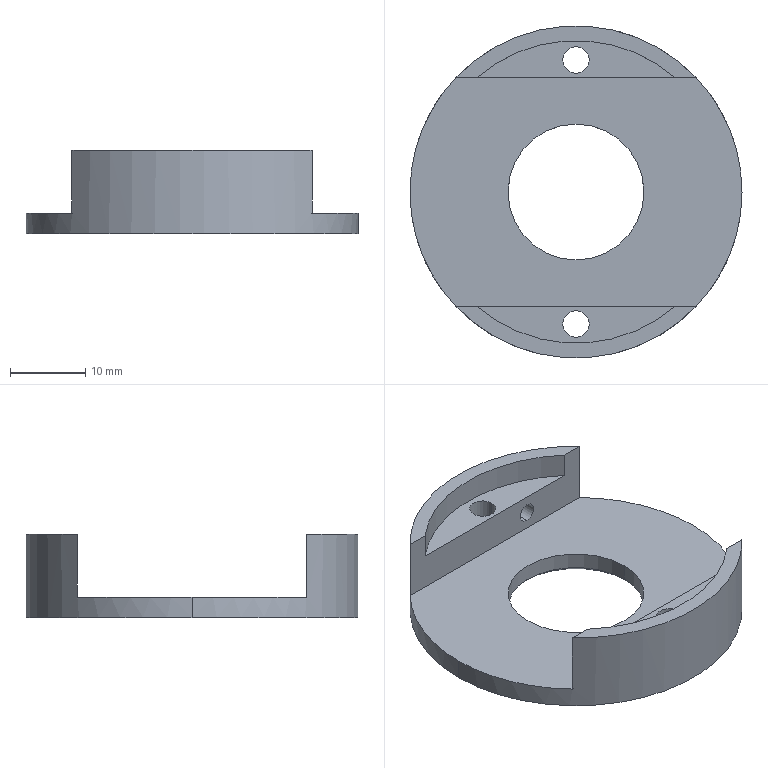Part | SolidWorks | features ICE 7, Chamfer 2, CirPattern 1, Extrusion 1 | 1 solid | 26 faces | box 44 x 44 x 11 mm | volume 5108 mm3 | cylinder 12 | plane 8 | cone 6 | commonest cylinder face diameters 3.5 x4 2.5 x2 18 x2 40.1 x2 44 x2
STEP:
#1=CARTESIAN_POINT('',(6.,21.166,6.45));
#2=VERTEX_POINT('',#1);
#3=CARTESIAN_POINT('',(6.,21.166,3.95));
#4=VERTEX_POINT('',#3);
#5=CARTESIAN_POINT('',(6.,21.166,6.45));
#6=CARTESIAN_POINT('',(5.841,21.211,6.45));
#7=CARTESIAN_POINT('',(5.679,21.255,6.419));
#8=CARTESIAN_POINT('',(5.381,21.332,6.298));
#9=CARTESIAN_POINT('',(5.241,21.367,6.207));
#10=CARTESIAN_POINT('',(5.009,21.423,5.979));
#11=CARTESIAN_POINT('',(4.913,21.444,5.839));
#12=CARTESIAN_POINT('',(4.817,21.466,5.611));
#13=CARTESIAN_POINT('',(4.792,21.472,5.53));
#14=CARTESIAN_POINT('',(4.759,21.479,5.368));
#15=CARTESIAN_POINT('',(4.75,21.481,5.285));
#16=CARTESIAN_POINT('',(4.75,21.481,5.035));
#17=CARTESIAN_POINT('',(4.783,21.474,4.87));
#18=CARTESIAN_POINT('',(4.88,21.452,4.639));
#19=CARTESIAN_POINT('',(4.919,21.443,4.567));
#20=CARTESIAN_POINT('',(5.011,21.422,4.431));
#21=CARTESIAN_POINT('',(5.065,21.409,4.367));
#22=CARTESIAN_POINT('',(5.24,21.367,4.194));
#23=CARTESIAN_POINT('',(5.379,21.333,4.103));
#24=CARTESIAN_POINT('',(5.677,21.255,3.982));
#25=CARTESIAN_POINT('',(5.839,21.212,3.95));
#26=CARTESIAN_POINT('',(6.,21.166,3.95));
#27=B_SPLINE_CURVE_WITH_KNOTS('',3,(#5,#6,#7,#8,#9,#10,#11,#12,#13,#14,#15,#16,#17,#18,#19,#20,#21,#22,#23,#24,#25,#26),.UNSPECIFIED.,.F.,.F.,(4,2,2,2,2,2,2,2,2,2,4),(0.003999,0.004495,0.004991,0.005487,0.005735,0.005983,0.006479,0.006727,0.006975,0.007471,0.007967),.UNSPECIFIED.);
#28=EDGE_CURVE('',#2,#4,#27,.T.);
#29=ORIENTED_EDGE('',*,*,#28,.F.);
#30=CARTESIAN_POINT('',(6.,15.2,6.45));
#31=VERTEX_POINT('',#30);
#32=CARTESIAN_POINT('',(6.,26.2,6.45));
#33=DIRECTION('',(0.,-1.,0.));
#34=VECTOR('',#33,1000.);
#35=LINE('',#32,#34);
#36=EDGE_CURVE('',#2,#31,#35,.T.);
#37=ORIENTED_EDGE('',*,*,#36,.T.);
#38=CARTESIAN_POINT('',(6.,15.2,3.95));
#39=VERTEX_POINT('',#38);
#40=CARTESIAN_POINT('',(6.,15.2,5.2));
#41=DIRECTION('',(0.,-1.,0.));
#42=DIRECTION('',(0.,0.,-1.));
#43=AXIS2_PLACEMENT_3D('',#40,#41,#42);
#44=CIRCLE('',#43,1.25);
#45=EDGE_CURVE('',#31,#39,#44,.T.);
#46=ORIENTED_EDGE('',*,*,#45,.T.);
#47=CARTESIAN_POINT('',(6.,26.2,3.95));
#48=DIRECTION('',(0.,-1.,0.));
#49=VECTOR('',#48,1000.);
#50=LINE('',#47,#49);
#51=EDGE_CURVE('',#4,#39,#50,.T.);
#52=ORIENTED_EDGE('',*,*,#51,.F.);
#53=EDGE_LOOP('',(#29,#37,#46,#52));
#54=FACE_OUTER_BOUND('',#53,.T.);
#55=CARTESIAN_POINT('',(6.,26.2,5.2));
#56=DIRECTION('',(0.,-1.,0.));
#57=DIRECTION('',(0.,0.,-1.));
#58=AXIS2_PLACEMENT_3D('',#55,#56,#57);
#59=CYLINDRICAL_SURFACE('',#58,1.25);
#60=ADVANCED_FACE('',(#54),#59,.F.);
#61=CARTESIAN_POINT('',(9.,0.,0.5));
#62=VERTEX_POINT('',#61);
#63=CARTESIAN_POINT('',(-9.,0.,0.5));
#64=VERTEX_POINT('',#63);
#65=CARTESIAN_POINT('',(0.,0.,0.5));
#66=DIRECTION('',(0.,0.,-1.));
#67=DIRECTION('',(1.,0.,0.));
#68=AXIS2_PLACEMENT_3D('',#65,#66,#67);
#69=CIRCLE('',#68,9.);
#70=EDGE_CURVE('',#62,#64,#69,.T.);
#71=ORIENTED_EDGE('',*,*,#70,.F.);
#72=CARTESIAN_POINT('',(9.5,0.,0.));
#73=VERTEX_POINT('',#72);
#74=CARTESIAN_POINT('',(9.,0.,0.5));
#75=DIRECTION('',(0.7071,0.,-0.7071));
#76=VECTOR('',#75,1000.);
#77=LINE('',#74,#76);
#78=EDGE_CURVE('',#62,#73,#77,.T.);
#79=ORIENTED_EDGE('',*,*,#78,.T.);
#80=CARTESIAN_POINT('',(-9.5,0.,0.));
#81=VERTEX_POINT('',#80);
#82=CARTESIAN_POINT('',(0.,0.,0.));
#83=DIRECTION('',(0.,0.,1.));
#84=DIRECTION('',(1.,0.,0.));
#85=AXIS2_PLACEMENT_3D('',#82,#83,#84);
#86=CIRCLE('',#85,9.5);
#87=EDGE_CURVE('',#81,#73,#86,.T.);
#88=ORIENTED_EDGE('',*,*,#87,.F.);
#89=CARTESIAN_POINT('',(-9.,0.,0.5));
#90=DIRECTION('',(-0.7071,0.,-0.7071));
#91=VECTOR('',#90,1000.);
#92=LINE('',#89,#91);
#93=EDGE_CURVE('',#64,#81,#92,.T.);
#94=ORIENTED_EDGE('',*,*,#93,.F.);
#95=EDGE_LOOP('',(#71,#79,#88,#94));
#96=FACE_OUTER_BOUND('',#95,.T.);
#97=CARTESIAN_POINT('',(0.,0.,0.5));
#98=DIRECTION('',(0.,0.,-1.));
#99=DIRECTION('',(-1.,0.,0.));
#100=AXIS2_PLACEMENT_3D('',#97,#98,#99);
#101=CONICAL_SURFACE('',#100,9.,0.7854);
#102=ADVANCED_FACE('',(#96),#101,.F.);
#103=CARTESIAN_POINT('',(1.75,17.5,1.5));
#104=VERTEX_POINT('',#103);
#105=CARTESIAN_POINT('',(-1.75,17.5,1.5));
#106=VERTEX_POINT('',#105);
#107=CARTESIAN_POINT('',(0.,17.5,1.5));
#108=DIRECTION('',(0.,0.,-1.));
#109=DIRECTION('',(1.,0.,0.));
#110=AXIS2_PLACEMENT_3D('',#107,#108,#109);
#111=CIRCLE('',#110,1.75);
#112=EDGE_CURVE('',#104,#106,#111,.T.);
#113=ORIENTED_EDGE('',*,*,#112,.F.);
#114=CARTESIAN_POINT('',(3.25,17.5,0.));
#115=VERTEX_POINT('',#114);
#116=CARTESIAN_POINT('',(1.75,17.5,1.5));
#117=DIRECTION('',(0.7071,0.,-0.7071));
#118=VECTOR('',#117,1000.);
#119=LINE('',#116,#118);
#120=EDGE_CURVE('',#104,#115,#119,.T.);
#121=ORIENTED_EDGE('',*,*,#120,.T.);
#122=CARTESIAN_POINT('',(-3.25,17.5,0.));
#123=VERTEX_POINT('',#122);
#124=CARTESIAN_POINT('',(0.,17.5,0.));
#125=DIRECTION('',(0.,0.,1.));
#126=DIRECTION('',(1.,0.,0.));
#127=AXIS2_PLACEMENT_3D('',#124,#125,#126);
#128=CIRCLE('',#127,3.25);
#129=EDGE_CURVE('',#123,#115,#128,.T.);
#130=ORIENTED_EDGE('',*,*,#129,.F.);
#131=CARTESIAN_POINT('',(-1.75,17.5,1.5));
#132=DIRECTION('',(-0.7071,0.,-0.7071));
#133=VECTOR('',#132,1000.);
#134=LINE('',#131,#133);
#135=EDGE_CURVE('',#106,#123,#134,.T.);
#136=ORIENTED_EDGE('',*,*,#135,.F.);
#137=EDGE_LOOP('',(#113,#121,#130,#136));
#138=FACE_OUTER_BOUND('',#137,.T.);
#139=CARTESIAN_POINT('',(0.,17.5,1.5));
#140=DIRECTION('',(0.,0.,-1.));
#141=DIRECTION('',(-1.,0.,0.));
#142=AXIS2_PLACEMENT_3D('',#139,#140,#141);
#143=CONICAL_SURFACE('',#142,1.75,0.7854);
#144=ADVANCED_FACE('',(#138),#143,.F.);
#145=CARTESIAN_POINT('',(1.75,-17.5,1.5));
#146=VERTEX_POINT('',#145);
#147=CARTESIAN_POINT('',(-1.75,-17.5,1.5));
#148=VERTEX_POINT('',#147);
#149=CARTESIAN_POINT('',(0.,-17.5,1.5));
#150=DIRECTION('',(0.,0.,-1.));
#151=DIRECTION('',(1.,0.,0.));
#152=AXIS2_PLACEMENT_3D('',#149,#150,#151);
#153=CIRCLE('',#152,1.75);
#154=EDGE_CURVE('',#146,#148,#153,.T.);
#155=ORIENTED_EDGE('',*,*,#154,.F.);
#156=CARTESIAN_POINT('',(3.25,-17.5,0.));
#157=VERTEX_POINT('',#156);
#158=CARTESIAN_POINT('',(1.75,-17.5,1.5));
#159=DIRECTION('',(0.7071,0.,-0.7071));
#160=VECTOR('',#159,1000.);
#161=LINE('',#158,#160);
#162=EDGE_CURVE('',#146,#157,#161,.T.);
#163=ORIENTED_EDGE('',*,*,#162,.T.);
#164=CARTESIAN_POINT('',(-3.25,-17.5,0.));
#165=VERTEX_POINT('',#164);
#166=CARTESIAN_POINT('',(0.,-17.5,0.));
#167=DIRECTION('',(0.,0.,1.));
#168=DIRECTION('',(1.,0.,0.));
#169=AXIS2_PLACEMENT_3D('',#166,#167,#168);
#170=CIRCLE('',#169,3.25);
#171=EDGE_CURVE('',#165,#157,#170,.T.);
#172=ORIENTED_EDGE('',*,*,#171,.F.);
#173=CARTESIAN_POINT('',(-1.75,-17.5,1.5));
#174=DIRECTION('',(-0.7071,0.,-0.7071));
#175=VECTOR('',#174,1000.);
#176=LINE('',#173,#175);
#177=EDGE_CURVE('',#148,#165,#176,.T.);
#178=ORIENTED_EDGE('',*,*,#177,.F.);
#179=EDGE_LOOP('',(#155,#163,#172,#178));
#180=FACE_OUTER_BOUND('',#179,.T.);
#181=CARTESIAN_POINT('',(0.,-17.5,1.5));
#182=DIRECTION('',(0.,0.,-1.));
#183=DIRECTION('',(-1.,0.,0.));
#184=AXIS2_PLACEMENT_3D('',#181,#182,#183);
#185=CONICAL_SURFACE('',#184,1.75,0.7854);
#186=ADVANCED_FACE('',(#180),#185,.F.);
#187=CARTESIAN_POINT('',(9.,0.,2.7));
#188=VERTEX_POINT('',#187);
#189=CARTESIAN_POINT('',(-9.,0.,2.7));
#190=VERTEX_POINT('',#189);
#191=CARTESIAN_POINT('',(0.,0.,2.7));
#192=DIRECTION('',(0.,0.,-1.));
#193=DIRECTION('',(1.,0.,0.));
#194=AXIS2_PLACEMENT_3D('',#191,#192,#193);
#195=CIRCLE('',#194,9.);
#196=EDGE_CURVE('',#188,#190,#195,.T.);
#197=ORIENTED_EDGE('',*,*,#196,.F.);
#198=CARTESIAN_POINT('',(9.,0.,11.001));
#199=DIRECTION('',(0.,0.,-1.));
#200=VECTOR('',#199,1000.);
#201=LINE('',#198,#200);
#202=EDGE_CURVE('',#188,#62,#201,.T.);
#203=ORIENTED_EDGE('',*,*,#202,.T.);
#204=ORIENTED_EDGE('',*,*,#70,.T.);
#205=CARTESIAN_POINT('',(-9.,0.,11.001));
#206=DIRECTION('',(0.,0.,-1.));
#207=VECTOR('',#206,1000.);
#208=LINE('',#205,#207);
#209=EDGE_CURVE('',#190,#64,#208,.T.);
#210=ORIENTED_EDGE('',*,*,#209,.F.);
#211=EDGE_LOOP('',(#197,#203,#204,#210));
#212=FACE_OUTER_BOUND('',#211,.T.);
#213=CARTESIAN_POINT('',(0.,0.,11.001));
#214=DIRECTION('',(0.,0.,-1.));
#215=DIRECTION('',(-1.,0.,0.));
#216=AXIS2_PLACEMENT_3D('',#213,#214,#215);
#217=CYLINDRICAL_SURFACE('',#216,9.);
#218=ADVANCED_FACE('',(#212),#217,.F.);
#219=CARTESIAN_POINT('',(-1.75,-17.5,7.7));
#220=VERTEX_POINT('',#219);
#221=CARTESIAN_POINT('',(1.75,-17.5,7.7));
#222=VERTEX_POINT('',#221);
#223=CARTESIAN_POINT('',(0.,-17.5,7.7));
#224=DIRECTION('',(0.,0.,1.));
#225=DIRECTION('',(1.,0.,0.));
#226=AXIS2_PLACEMENT_3D('',#223,#224,#225);
#227=CIRCLE('',#226,1.75);
#228=EDGE_CURVE('',#220,#222,#227,.T.);
#229=ORIENTED_EDGE('',*,*,#228,.T.);
#230=CARTESIAN_POINT('',(1.75,-17.5,5.));
#231=DIRECTION('',(0.,0.,-1.));
#232=VECTOR('',#231,1000.);
#233=LINE('',#230,#232);
#234=EDGE_CURVE('',#222,#146,#233,.T.);
#235=ORIENTED_EDGE('',*,*,#234,.T.);
#236=ORIENTED_EDGE('',*,*,#154,.T.);
#237=CARTESIAN_POINT('',(-1.75,-17.5,5.));
#238=DIRECTION('',(0.,0.,-1.));
#239=VECTOR('',#238,1000.);
#240=LINE('',#237,#239);
#241=EDGE_CURVE('',#220,#148,#240,.T.);
#242=ORIENTED_EDGE('',*,*,#241,.F.);
#243=EDGE_LOOP('',(#229,#235,#236,#242));
#244=FACE_OUTER_BOUND('',#243,.T.);
#245=CARTESIAN_POINT('',(0.,-17.5,5.));
#246=DIRECTION('',(0.,0.,-1.));
#247=DIRECTION('',(-1.,0.,0.));
#248=AXIS2_PLACEMENT_3D('',#245,#246,#247);
#249=CYLINDRICAL_SURFACE('',#248,1.75);
#250=ADVANCED_FACE('',(#244),#249,.F.);
#251=CARTESIAN_POINT('',(-1.75,17.5,7.7));
#252=VERTEX_POINT('',#251);
#253=CARTESIAN_POINT('',(1.75,17.5,7.7));
#254=VERTEX_POINT('',#253);
#255=CARTESIAN_POINT('',(0.,17.5,7.7));
#256=DIRECTION('',(0.,0.,1.));
#257=DIRECTION('',(1.,0.,0.));
#258=AXIS2_PLACEMENT_3D('',#255,#256,#257);
#259=CIRCLE('',#258,1.75);
#260=EDGE_CURVE('',#252,#254,#259,.T.);
#261=ORIENTED_EDGE('',*,*,#260,.T.);
#262=CARTESIAN_POINT('',(1.75,17.5,5.));
#263=DIRECTION('',(0.,0.,-1.));
#264=VECTOR('',#263,1000.);
#265=LINE('',#262,#264);
#266=EDGE_CURVE('',#254,#104,#265,.T.);
#267=ORIENTED_EDGE('',*,*,#266,.T.);
#268=ORIENTED_EDGE('',*,*,#112,.T.);
#269=CARTESIAN_POINT('',(-1.75,17.5,5.));
#270=DIRECTION('',(0.,0.,-1.));
#271=VECTOR('',#270,1000.);
#272=LINE('',#269,#271);
#273=EDGE_CURVE('',#252,#106,#272,.T.);
#274=ORIENTED_EDGE('',*,*,#273,.F.);
#275=EDGE_LOOP('',(#261,#267,#268,#274));
#276=FACE_OUTER_BOUND('',#275,.T.);
#277=CARTESIAN_POINT('',(0.,17.5,5.));
#278=DIRECTION('',(0.,0.,-1.));
#279=DIRECTION('',(-1.,0.,0.));
#280=AXIS2_PLACEMENT_3D('',#277,#278,#279);
#281=CYLINDRICAL_SURFACE('',#280,1.75);
#282=ADVANCED_FACE('',(#276),#281,.F.);
#283=CARTESIAN_POINT('',(6.,21.166,3.95));
#284=CARTESIAN_POINT('',(6.163,21.12,3.95));
#285=CARTESIAN_POINT('',(6.321,21.073,3.981));
#286=CARTESIAN_POINT('',(6.621,20.981,4.103));
#287=CARTESIAN_POINT('',(6.758,20.937,4.193));
#288=CARTESIAN_POINT('',(6.933,20.879,4.364));
#289=CARTESIAN_POINT('',(6.985,20.862,4.426));
#290=CARTESIAN_POINT('',(7.078,20.83,4.562));
#291=CARTESIAN_POINT('',(7.118,20.817,4.635));
#292=CARTESIAN_POINT('',(7.215,20.783,4.864));
#293=CARTESIAN_POINT('',(7.25,20.771,5.032));
#294=CARTESIAN_POINT('',(7.25,20.771,5.365));
#295=CARTESIAN_POINT('',(7.216,20.783,5.533));
#296=CARTESIAN_POINT('',(7.087,20.827,5.84));
#297=CARTESIAN_POINT('',(6.992,20.86,5.978));
#298=CARTESIAN_POINT('',(6.758,20.937,6.208));
#299=CARTESIAN_POINT('',(6.62,20.981,6.297));
#300=CARTESIAN_POINT('',(6.322,21.073,6.419));
#301=CARTESIAN_POINT('',(6.161,21.12,6.45));
#302=CARTESIAN_POINT('',(6.,21.166,6.45));
#303=B_SPLINE_CURVE_WITH_KNOTS('',3,(#283,#284,#285,#286,#287,#288,#289,#290,#291,#292,#293,#294,#295,#296,#297,#298,#299,#300,#301,#302),.UNSPECIFIED.,.F.,.F.,(4,2,2,2,2,2,2,2,2,4),(0.,0.0004999,0.0009998,0.00125,0.0015,0.002,0.002499,0.002999,0.003499,0.003999),.UNSPECIFIED.);
#304=EDGE_CURVE('',#4,#2,#303,.T.);
#305=ORIENTED_EDGE('',*,*,#304,.T.);
#306=ORIENTED_EDGE('',*,*,#28,.T.);
#307=EDGE_LOOP('',(#305,#306));
#308=FACE_BOUND('',#307,.T.);
#309=CARTESIAN_POINT('',(22.,0.,2.7));
#310=VERTEX_POINT('',#309);
#311=CARTESIAN_POINT('',(15.905,15.2,2.7));
#312=VERTEX_POINT('',#311);
#313=CARTESIAN_POINT('',(0.,0.,2.7));
#314=DIRECTION('',(0.,0.,1.));
#315=DIRECTION('',(1.,0.,0.));
#316=AXIS2_PLACEMENT_3D('',#313,#314,#315);
#317=CIRCLE('',#316,22.);
#318=EDGE_CURVE('',#310,#312,#317,.T.);
#319=ORIENTED_EDGE('',*,*,#318,.F.);
#320=CARTESIAN_POINT('',(22.,0.,0.));
#321=VERTEX_POINT('',#320);
#322=CARTESIAN_POINT('',(22.,0.,11.));
#323=DIRECTION('',(0.,0.,-1.));
#324=VECTOR('',#323,1000.);
#325=LINE('',#322,#324);
#326=EDGE_CURVE('',#310,#321,#325,.T.);
#327=ORIENTED_EDGE('',*,*,#326,.T.);
#328=CARTESIAN_POINT('',(-22.,0.,0.));
#329=VERTEX_POINT('',#328);
#330=CARTESIAN_POINT('',(0.,0.,0.));
#331=DIRECTION('',(0.,0.,1.));
#332=DIRECTION('',(1.,0.,0.));
#333=AXIS2_PLACEMENT_3D('',#330,#331,#332);
#334=CIRCLE('',#333,22.);
#335=EDGE_CURVE('',#321,#329,#334,.T.);
#336=ORIENTED_EDGE('',*,*,#335,.T.);
#337=CARTESIAN_POINT('',(-22.,0.,2.7));
#338=VERTEX_POINT('',#337);
#339=CARTESIAN_POINT('',(-22.,0.,11.));
#340=DIRECTION('',(0.,0.,-1.));
#341=VECTOR('',#340,1000.);
#342=LINE('',#339,#341);
#343=EDGE_CURVE('',#338,#329,#342,.T.);
#344=ORIENTED_EDGE('',*,*,#343,.F.);
#345=CARTESIAN_POINT('',(-15.905,15.2,2.7));
#346=VERTEX_POINT('',#345);
#347=CARTESIAN_POINT('',(0.,0.,2.7));
#348=DIRECTION('',(0.,0.,1.));
#349=DIRECTION('',(1.,0.,0.));
#350=AXIS2_PLACEMENT_3D('',#347,#348,#349);
#351=CIRCLE('',#350,22.);
#352=EDGE_CURVE('',#346,#338,#351,.T.);
#353=ORIENTED_EDGE('',*,*,#352,.F.);
#354=CARTESIAN_POINT('',(-15.905,15.2,11.));
#355=VERTEX_POINT('',#354);
#356=CARTESIAN_POINT('',(-15.905,15.2,11.));
#357=DIRECTION('',(0.,0.,-1.));
#358=VECTOR('',#357,1000.);
#359=LINE('',#356,#358);
#360=EDGE_CURVE('',#355,#346,#359,.T.);
#361=ORIENTED_EDGE('',*,*,#360,.F.);
#362=CARTESIAN_POINT('',(15.905,15.2,11.));
#363=VERTEX_POINT('',#362);
#364=CARTESIAN_POINT('',(0.,0.,11.));
#365=DIRECTION('',(0.,0.,1.));
#366=DIRECTION('',(1.,0.,0.));
#367=AXIS2_PLACEMENT_3D('',#364,#365,#366);
#368=CIRCLE('',#367,22.);
#369=EDGE_CURVE('',#363,#355,#368,.T.);
#370=ORIENTED_EDGE('',*,*,#369,.F.);
#371=CARTESIAN_POINT('',(15.905,15.2,11.));
#372=DIRECTION('',(0.,0.,1.));
#373=VECTOR('',#372,1000.);
#374=LINE('',#371,#373);
#375=EDGE_CURVE('',#312,#363,#374,.T.);
#376=ORIENTED_EDGE('',*,*,#375,.F.);
#377=EDGE_LOOP('',(#319,#327,#336,#344,#353,#361,#370,#376));
#378=FACE_OUTER_BOUND('',#377,.T.);
#379=CARTESIAN_POINT('',(0.,0.,11.));
#380=DIRECTION('',(0.,0.,-1.));
#381=DIRECTION('',(-1.,0.,0.));
#382=AXIS2_PLACEMENT_3D('',#379,#380,#381);
#383=CYLINDRICAL_SURFACE('',#382,22.);
#384=ADVANCED_FACE('',(#308,#378),#383,.T.);
#385=CARTESIAN_POINT('',(0.,0.,2.7));
#386=DIRECTION('',(0.,0.,-1.));
#387=DIRECTION('',(1.,0.,0.));
#388=AXIS2_PLACEMENT_3D('',#385,#386,#387);
#389=CIRCLE('',#388,9.);
#390=EDGE_CURVE('',#190,#188,#389,.T.);
#391=ORIENTED_EDGE('',*,*,#390,.T.);
#392=ORIENTED_EDGE('',*,*,#196,.T.);
#393=EDGE_LOOP('',(#391,#392));
#394=FACE_BOUND('',#393,.T.);
#395=CARTESIAN_POINT('',(15.905,-15.2,2.7));
#396=VERTEX_POINT('',#395);
#397=CARTESIAN_POINT('',(0.,0.,2.7));
#398=DIRECTION('',(0.,0.,1.));
#399=DIRECTION('',(1.,0.,0.));
#400=AXIS2_PLACEMENT_3D('',#397,#398,#399);
#401=CIRCLE('',#400,22.);
#402=EDGE_CURVE('',#396,#310,#401,.T.);
#403=ORIENTED_EDGE('',*,*,#402,.T.);
#404=ORIENTED_EDGE('',*,*,#318,.T.);
#405=CARTESIAN_POINT('',(-33.841,15.2,2.7));
#406=DIRECTION('',(-1.,0.,0.));
#407=VECTOR('',#406,1000.);
#408=LINE('',#405,#407);
#409=EDGE_CURVE('',#312,#346,#408,.T.);
#410=ORIENTED_EDGE('',*,*,#409,.T.);
#411=ORIENTED_EDGE('',*,*,#352,.T.);
#412=CARTESIAN_POINT('',(-15.905,-15.2,2.7));
#413=VERTEX_POINT('',#412);
#414=CARTESIAN_POINT('',(0.,0.,2.7));
#415=DIRECTION('',(0.,0.,1.));
#416=DIRECTION('',(1.,0.,0.));
#417=AXIS2_PLACEMENT_3D('',#414,#415,#416);
#418=CIRCLE('',#417,22.);
#419=EDGE_CURVE('',#338,#413,#418,.T.);
#420=ORIENTED_EDGE('',*,*,#419,.T.);
#421=CARTESIAN_POINT('',(-33.841,-15.2,2.7));
#422=DIRECTION('',(1.,0.,0.));
#423=VECTOR('',#422,1000.);
#424=LINE('',#421,#423);
#425=EDGE_CURVE('',#413,#396,#424,.T.);
#426=ORIENTED_EDGE('',*,*,#425,.T.);
#427=EDGE_LOOP('',(#403,#404,#410,#411,#420,#426));
#428=FACE_OUTER_BOUND('',#427,.T.);
#429=CARTESIAN_POINT('',(0.,0.,2.7));
#430=DIRECTION('',(0.,0.,1.));
#431=DIRECTION('',(1.,0.,0.));
#432=AXIS2_PLACEMENT_3D('',#429,#430,#431);
#433=PLANE('',#432);
#434=ADVANCED_FACE('',(#394,#428),#433,.T.);
#435=ORIENTED_EDGE('',*,*,#326,.F.);
#436=ORIENTED_EDGE('',*,*,#402,.F.);
#437=CARTESIAN_POINT('',(15.905,-15.2,11.));
#438=VERTEX_POINT('',#437);
#439=CARTESIAN_POINT('',(15.905,-15.2,11.));
#440=DIRECTION('',(0.,0.,-1.));
#441=VECTOR('',#440,1000.);
#442=LINE('',#439,#441);
#443=EDGE_CURVE('',#438,#396,#442,.T.);
#444=ORIENTED_EDGE('',*,*,#443,.F.);
#445=CARTESIAN_POINT('',(-15.905,-15.2,11.));
#446=VERTEX_POINT('',#445);
#447=CARTESIAN_POINT('',(0.,0.,11.));
#448=DIRECTION('',(0.,0.,1.));
#449=DIRECTION('',(1.,0.,0.));
#450=AXIS2_PLACEMENT_3D('',#447,#448,#449);
#451=CIRCLE('',#450,22.);
#452=EDGE_CURVE('',#446,#438,#451,.T.);
#453=ORIENTED_EDGE('',*,*,#452,.F.);
#454=CARTESIAN_POINT('',(-15.905,-15.2,11.));
#455=DIRECTION('',(0.,0.,1.));
#456=VECTOR('',#455,1000.);
#457=LINE('',#454,#456);
#458=EDGE_CURVE('',#413,#446,#457,.T.);
#459=ORIENTED_EDGE('',*,*,#458,.F.);
#460=ORIENTED_EDGE('',*,*,#419,.F.);
#461=ORIENTED_EDGE('',*,*,#343,.T.);
#462=CARTESIAN_POINT('',(0.,0.,0.));
#463=DIRECTION('',(0.,0.,1.));
#464=DIRECTION('',(1.,0.,0.));
#465=AXIS2_PLACEMENT_3D('',#462,#463,#464);
#466=CIRCLE('',#465,22.);
#467=EDGE_CURVE('',#329,#321,#466,.T.);
#468=ORIENTED_EDGE('',*,*,#467,.T.);
#469=EDGE_LOOP('',(#435,#436,#444,#453,#459,#460,#461,#468));
#470=FACE_OUTER_BOUND('',#469,.T.);
#471=CARTESIAN_POINT('',(0.,0.,11.));
#472=DIRECTION('',(0.,0.,-1.));
#473=DIRECTION('',(-1.,0.,0.));
#474=AXIS2_PLACEMENT_3D('',#471,#472,#473);
#475=CYLINDRICAL_SURFACE('',#474,22.);
#476=ADVANCED_FACE('',(#470),#475,.T.);
#477=ORIENTED_EDGE('',*,*,#369,.T.);
#478=CARTESIAN_POINT('',(-13.075,15.2,11.));
#479=VERTEX_POINT('',#478);
#480=CARTESIAN_POINT('',(-33.841,15.2,11.));
#481=DIRECTION('',(-1.,0.,0.));
#482=VECTOR('',#481,1000.);
#483=LINE('',#480,#482);
#484=EDGE_CURVE('',#479,#355,#483,.T.);
#485=ORIENTED_EDGE('',*,*,#484,.F.);
#486=CARTESIAN_POINT('',(13.075,15.2,11.));
#487=VERTEX_POINT('',#486);
#488=CARTESIAN_POINT('',(0.,0.,11.));
#489=DIRECTION('',(0.,0.,1.));
#490=DIRECTION('',(1.,0.,0.));
#491=AXIS2_PLACEMENT_3D('',#488,#489,#490);
#492=CIRCLE('',#491,20.05);
#493=EDGE_CURVE('',#487,#479,#492,.T.);
#494=ORIENTED_EDGE('',*,*,#493,.F.);
#495=CARTESIAN_POINT('',(-33.841,15.2,11.));
#496=DIRECTION('',(-1.,0.,0.));
#497=VECTOR('',#496,1000.);
#498=LINE('',#495,#497);
#499=EDGE_CURVE('',#363,#487,#498,.T.);
#500=ORIENTED_EDGE('',*,*,#499,.F.);
#501=EDGE_LOOP('',(#477,#485,#494,#500));
#502=FACE_OUTER_BOUND('',#501,.T.);
#503=CARTESIAN_POINT('',(0.,0.,11.));
#504=DIRECTION('',(0.,0.,1.));
#505=DIRECTION('',(1.,0.,0.));
#506=AXIS2_PLACEMENT_3D('',#503,#504,#505);
#507=PLANE('',#506);
#508=ADVANCED_FACE('',(#502),#507,.T.);
#509=ORIENTED_EDGE('',*,*,#452,.T.);
#510=CARTESIAN_POINT('',(13.075,-15.2,11.));
#511=VERTEX_POINT('',#510);
#512=CARTESIAN_POINT('',(-33.841,-15.2,11.));
#513=DIRECTION('',(1.,0.,0.));
#514=VECTOR('',#513,1000.);
#515=LINE('',#512,#514);
#516=EDGE_CURVE('',#511,#438,#515,.T.);
#517=ORIENTED_EDGE('',*,*,#516,.F.);
#518=CARTESIAN_POINT('',(-13.075,-15.2,11.));
#519=VERTEX_POINT('',#518);
#520=CARTESIAN_POINT('',(0.,0.,11.));
#521=DIRECTION('',(0.,0.,1.));
#522=DIRECTION('',(1.,0.,0.));
#523=AXIS2_PLACEMENT_3D('',#520,#521,#522);
#524=CIRCLE('',#523,20.05);
#525=EDGE_CURVE('',#519,#511,#524,.T.);
#526=ORIENTED_EDGE('',*,*,#525,.F.);
#527=CARTESIAN_POINT('',(-33.841,-15.2,11.));
#528=DIRECTION('',(1.,0.,0.));
#529=VECTOR('',#528,1000.);
#530=LINE('',#527,#529);
#531=EDGE_CURVE('',#446,#519,#530,.T.);
#532=ORIENTED_EDGE('',*,*,#531,.F.);
#533=EDGE_LOOP('',(#509,#517,#526,#532));
#534=FACE_OUTER_BOUND('',#533,.T.);
#535=CARTESIAN_POINT('',(0.,0.,11.));
#536=DIRECTION('',(0.,0.,1.));
#537=DIRECTION('',(1.,0.,0.));
#538=AXIS2_PLACEMENT_3D('',#535,#536,#537);
#539=PLANE('',#538);
#540=ADVANCED_FACE('',(#534),#539,.T.);
#541=CARTESIAN_POINT('',(-13.075,15.2,7.7));
#542=VERTEX_POINT('',#541);
#543=CARTESIAN_POINT('',(-13.075,15.2,2.7));
#544=DIRECTION('',(0.,0.,1.));
#545=VECTOR('',#544,1000.);
#546=LINE('',#543,#545);
#547=EDGE_CURVE('',#542,#479,#546,.T.);
#548=ORIENTED_EDGE('',*,*,#547,.F.);
#549=CARTESIAN_POINT('',(13.075,15.2,7.7));
#550=VERTEX_POINT('',#549);
#551=CARTESIAN_POINT('',(0.,0.,7.7));
#552=DIRECTION('',(0.,0.,1.));
#553=DIRECTION('',(1.,0.,0.));
#554=AXIS2_PLACEMENT_3D('',#551,#552,#553);
#555=CIRCLE('',#554,20.05);
#556=EDGE_CURVE('',#550,#542,#555,.T.);
#557=ORIENTED_EDGE('',*,*,#556,.F.);
#558=CARTESIAN_POINT('',(13.075,15.2,2.7));
#559=DIRECTION('',(0.,0.,-1.));
#560=VECTOR('',#559,1000.);
#561=LINE('',#558,#560);
#562=EDGE_CURVE('',#487,#550,#561,.T.);
#563=ORIENTED_EDGE('',*,*,#562,.F.);
#564=ORIENTED_EDGE('',*,*,#493,.T.);
#565=EDGE_LOOP('',(#548,#557,#563,#564));
#566=FACE_OUTER_BOUND('',#565,.T.);
#567=CARTESIAN_POINT('',(0.,0.,2.7));
#568=DIRECTION('',(0.,0.,1.));
#569=DIRECTION('',(1.,0.,0.));
#570=AXIS2_PLACEMENT_3D('',#567,#568,#569);
#571=CYLINDRICAL_SURFACE('',#570,20.05);
#572=ADVANCED_FACE('',(#566),#571,.F.);
#573=CARTESIAN_POINT('',(13.075,-15.2,7.7));
#574=VERTEX_POINT('',#573);
#575=CARTESIAN_POINT('',(13.075,-15.2,2.7));
#576=DIRECTION('',(0.,0.,1.));
#577=VECTOR('',#576,1000.);
#578=LINE('',#575,#577);
#579=EDGE_CURVE('',#574,#511,#578,.T.);
#580=ORIENTED_EDGE('',*,*,#579,.F.);
#581=CARTESIAN_POINT('',(-13.075,-15.2,7.7));
#582=VERTEX_POINT('',#581);
#583=CARTESIAN_POINT('',(0.,0.,7.7));
#584=DIRECTION('',(0.,0.,1.));
#585=DIRECTION('',(1.,0.,0.));
#586=AXIS2_PLACEMENT_3D('',#583,#584,#585);
#587=CIRCLE('',#586,20.05);
#588=EDGE_CURVE('',#582,#574,#587,.T.);
#589=ORIENTED_EDGE('',*,*,#588,.F.);
#590=CARTESIAN_POINT('',(-13.075,-15.2,2.7));
#591=DIRECTION('',(0.,0.,-1.));
#592=VECTOR('',#591,1000.);
#593=LINE('',#590,#592);
#594=EDGE_CURVE('',#519,#582,#593,.T.);
#595=ORIENTED_EDGE('',*,*,#594,.F.);
#596=ORIENTED_EDGE('',*,*,#525,.T.);
#597=EDGE_LOOP('',(#580,#589,#595,#596));
#598=FACE_OUTER_BOUND('',#597,.T.);
#599=CARTESIAN_POINT('',(0.,0.,2.7));
#600=DIRECTION('',(0.,0.,1.));
#601=DIRECTION('',(1.,0.,0.));
#602=AXIS2_PLACEMENT_3D('',#599,#600,#601);
#603=CYLINDRICAL_SURFACE('',#602,20.05);
#604=ADVANCED_FACE('',(#598),#603,.F.);
#605=ORIENTED_EDGE('',*,*,#87,.T.);
#606=CARTESIAN_POINT('',(0.,0.,0.));
#607=DIRECTION('',(0.,0.,1.));
#608=DIRECTION('',(1.,0.,0.));
#609=AXIS2_PLACEMENT_3D('',#606,#607,#608);
#610=CIRCLE('',#609,9.5);
#611=EDGE_CURVE('',#73,#81,#610,.T.);
#612=ORIENTED_EDGE('',*,*,#611,.T.);
#613=EDGE_LOOP('',(#605,#612));
#614=FACE_BOUND('',#613,.T.);
#615=ORIENTED_EDGE('',*,*,#171,.T.);
#616=CARTESIAN_POINT('',(0.,-17.5,0.));
#617=DIRECTION('',(0.,0.,1.));
#618=DIRECTION('',(1.,0.,0.));
#619=AXIS2_PLACEMENT_3D('',#616,#617,#618);
#620=CIRCLE('',#619,3.25);
#621=EDGE_CURVE('',#157,#165,#620,.T.);
#622=ORIENTED_EDGE('',*,*,#621,.T.);
#623=EDGE_LOOP('',(#615,#622));
#624=FACE_BOUND('',#623,.T.);
#625=ORIENTED_EDGE('',*,*,#129,.T.);
#626=CARTESIAN_POINT('',(0.,17.5,0.));
#627=DIRECTION('',(0.,0.,1.));
#628=DIRECTION('',(1.,0.,0.));
#629=AXIS2_PLACEMENT_3D('',#626,#627,#628);
#630=CIRCLE('',#629,3.25);
#631=EDGE_CURVE('',#115,#123,#630,.T.);
#632=ORIENTED_EDGE('',*,*,#631,.T.);
#633=EDGE_LOOP('',(#625,#632));
#634=FACE_BOUND('',#633,.T.);
#635=ORIENTED_EDGE('',*,*,#467,.F.);
#636=ORIENTED_EDGE('',*,*,#335,.F.);
#637=EDGE_LOOP('',(#635,#636));
#638=FACE_OUTER_BOUND('',#637,.T.);
#639=CARTESIAN_POINT('',(0.,0.,0.));
#640=DIRECTION('',(0.,0.,1.));
#641=DIRECTION('',(1.,0.,0.));
#642=AXIS2_PLACEMENT_3D('',#639,#640,#641);
#643=PLANE('',#642);
#644=ADVANCED_FACE('',(#614,#624,#634,#638),#643,.F.);
#645=ORIENTED_EDGE('',*,*,#443,.T.);
#646=ORIENTED_EDGE('',*,*,#425,.F.);
#647=ORIENTED_EDGE('',*,*,#458,.T.);
#648=ORIENTED_EDGE('',*,*,#531,.T.);
#649=ORIENTED_EDGE('',*,*,#594,.T.);
#650=CARTESIAN_POINT('',(-13.075,-15.2,7.7));
#651=DIRECTION('',(-1.,0.,0.));
#652=VECTOR('',#651,1000.);
#653=LINE('',#650,#652);
#654=EDGE_CURVE('',#574,#582,#653,.T.);
#655=ORIENTED_EDGE('',*,*,#654,.F.);
#656=ORIENTED_EDGE('',*,*,#579,.T.);
#657=ORIENTED_EDGE('',*,*,#516,.T.);
#658=EDGE_LOOP('',(#645,#646,#647,#648,#649,#655,#656,#657));
#659=FACE_OUTER_BOUND('',#658,.T.);
#660=CARTESIAN_POINT('',(-33.841,-15.2,85.197));
#661=DIRECTION('',(0.,1.,0.));
#662=DIRECTION('',(0.,0.,1.));
#663=AXIS2_PLACEMENT_3D('',#660,#661,#662);
#664=PLANE('',#663);
#665=ADVANCED_FACE('',(#659),#664,.T.);
#666=CARTESIAN_POINT('',(6.,15.2,5.2));
#667=DIRECTION('',(0.,-1.,0.));
#668=DIRECTION('',(0.,0.,-1.));
#669=AXIS2_PLACEMENT_3D('',#666,#667,#668);
#670=CIRCLE('',#669,1.25);
#671=EDGE_CURVE('',#39,#31,#670,.T.);
#672=ORIENTED_EDGE('',*,*,#671,.F.);
#673=ORIENTED_EDGE('',*,*,#45,.F.);
#674=EDGE_LOOP('',(#672,#673));
#675=FACE_BOUND('',#674,.T.);
#676=ORIENTED_EDGE('',*,*,#360,.T.);
#677=ORIENTED_EDGE('',*,*,#409,.F.);
#678=ORIENTED_EDGE('',*,*,#375,.T.);
#679=ORIENTED_EDGE('',*,*,#499,.T.);
#680=ORIENTED_EDGE('',*,*,#562,.T.);
#681=CARTESIAN_POINT('',(-13.075,15.2,7.7));
#682=DIRECTION('',(1.,0.,0.));
#683=VECTOR('',#682,1000.);
#684=LINE('',#681,#683);
#685=EDGE_CURVE('',#542,#550,#684,.T.);
#686=ORIENTED_EDGE('',*,*,#685,.F.);
#687=ORIENTED_EDGE('',*,*,#547,.T.);
#688=ORIENTED_EDGE('',*,*,#484,.T.);
#689=EDGE_LOOP('',(#676,#677,#678,#679,#680,#686,#687,#688));
#690=FACE_OUTER_BOUND('',#689,.T.);
#691=CARTESIAN_POINT('',(-33.841,15.2,85.197));
#692=DIRECTION('',(0.,-1.,0.));
#693=DIRECTION('',(0.,0.,-1.));
#694=AXIS2_PLACEMENT_3D('',#691,#692,#693);
#695=PLANE('',#694);
#696=ADVANCED_FACE('',(#675,#690),#695,.T.);
#697=ORIENTED_EDGE('',*,*,#266,.F.);
#698=CARTESIAN_POINT('',(0.,17.5,7.7));
#699=DIRECTION('',(0.,0.,1.));
#700=DIRECTION('',(1.,0.,0.));
#701=AXIS2_PLACEMENT_3D('',#698,#699,#700);
#702=CIRCLE('',#701,1.75);
#703=EDGE_CURVE('',#254,#252,#702,.T.);
#704=ORIENTED_EDGE('',*,*,#703,.T.);
#705=ORIENTED_EDGE('',*,*,#273,.T.);
#706=CARTESIAN_POINT('',(0.,17.5,1.5));
#707=DIRECTION('',(0.,0.,-1.));
#708=DIRECTION('',(1.,0.,0.));
#709=AXIS2_PLACEMENT_3D('',#706,#707,#708);
#710=CIRCLE('',#709,1.75);
#711=EDGE_CURVE('',#106,#104,#710,.T.);
#712=ORIENTED_EDGE('',*,*,#711,.T.);
#713=EDGE_LOOP('',(#697,#704,#705,#712));
#714=FACE_OUTER_BOUND('',#713,.T.);
#715=CARTESIAN_POINT('',(0.,17.5,5.));
#716=DIRECTION('',(0.,0.,-1.));
#717=DIRECTION('',(-1.,0.,0.));
#718=AXIS2_PLACEMENT_3D('',#715,#716,#717);
#719=CYLINDRICAL_SURFACE('',#718,1.75);
#720=ADVANCED_FACE('',(#714),#719,.F.);
#721=ORIENTED_EDGE('',*,*,#234,.F.);
#722=CARTESIAN_POINT('',(0.,-17.5,7.7));
#723=DIRECTION('',(0.,0.,1.));
#724=DIRECTION('',(1.,0.,0.));
#725=AXIS2_PLACEMENT_3D('',#722,#723,#724);
#726=CIRCLE('',#725,1.75);
#727=EDGE_CURVE('',#222,#220,#726,.T.);
#728=ORIENTED_EDGE('',*,*,#727,.T.);
#729=ORIENTED_EDGE('',*,*,#241,.T.);
#730=CARTESIAN_POINT('',(0.,-17.5,1.5));
#731=DIRECTION('',(0.,0.,-1.));
#732=DIRECTION('',(1.,0.,0.));
#733=AXIS2_PLACEMENT_3D('',#730,#731,#732);
#734=CIRCLE('',#733,1.75);
#735=EDGE_CURVE('',#148,#146,#734,.T.);
#736=ORIENTED_EDGE('',*,*,#735,.T.);
#737=EDGE_LOOP('',(#721,#728,#729,#736));
#738=FACE_OUTER_BOUND('',#737,.T.);
#739=CARTESIAN_POINT('',(0.,-17.5,5.));
#740=DIRECTION('',(0.,0.,-1.));
#741=DIRECTION('',(-1.,0.,0.));
#742=AXIS2_PLACEMENT_3D('',#739,#740,#741);
#743=CYLINDRICAL_SURFACE('',#742,1.75);
#744=ADVANCED_FACE('',(#738),#743,.F.);
#745=ORIENTED_EDGE('',*,*,#202,.F.);
#746=ORIENTED_EDGE('',*,*,#390,.F.);
#747=ORIENTED_EDGE('',*,*,#209,.T.);
#748=CARTESIAN_POINT('',(0.,0.,0.5));
#749=DIRECTION('',(0.,0.,-1.));
#750=DIRECTION('',(1.,0.,0.));
#751=AXIS2_PLACEMENT_3D('',#748,#749,#750);
#752=CIRCLE('',#751,9.);
#753=EDGE_CURVE('',#64,#62,#752,.T.);
#754=ORIENTED_EDGE('',*,*,#753,.T.);
#755=EDGE_LOOP('',(#745,#746,#747,#754));
#756=FACE_OUTER_BOUND('',#755,.T.);
#757=CARTESIAN_POINT('',(0.,0.,11.001));
#758=DIRECTION('',(0.,0.,-1.));
#759=DIRECTION('',(-1.,0.,0.));
#760=AXIS2_PLACEMENT_3D('',#757,#758,#759);
#761=CYLINDRICAL_SURFACE('',#760,9.);
#762=ADVANCED_FACE('',(#756),#761,.F.);
#763=ORIENTED_EDGE('',*,*,#162,.F.);
#764=ORIENTED_EDGE('',*,*,#735,.F.);
#765=ORIENTED_EDGE('',*,*,#177,.T.);
#766=ORIENTED_EDGE('',*,*,#621,.F.);
#767=EDGE_LOOP('',(#763,#764,#765,#766));
#768=FACE_OUTER_BOUND('',#767,.T.);
#769=CARTESIAN_POINT('',(0.,-17.5,1.5));
#770=DIRECTION('',(0.,0.,-1.));
#771=DIRECTION('',(-1.,0.,0.));
#772=AXIS2_PLACEMENT_3D('',#769,#770,#771);
#773=CONICAL_SURFACE('',#772,1.75,0.7854);
#774=ADVANCED_FACE('',(#768),#773,.F.);
#775=ORIENTED_EDGE('',*,*,#120,.F.);
#776=ORIENTED_EDGE('',*,*,#711,.F.);
#777=ORIENTED_EDGE('',*,*,#135,.T.);
#778=ORIENTED_EDGE('',*,*,#631,.F.);
#779=EDGE_LOOP('',(#775,#776,#777,#778));
#780=FACE_OUTER_BOUND('',#779,.T.);
#781=CARTESIAN_POINT('',(0.,17.5,1.5));
#782=DIRECTION('',(0.,0.,-1.));
#783=DIRECTION('',(-1.,0.,0.));
#784=AXIS2_PLACEMENT_3D('',#781,#782,#783);
#785=CONICAL_SURFACE('',#784,1.75,0.7854);
#786=ADVANCED_FACE('',(#780),#785,.F.);
#787=ORIENTED_EDGE('',*,*,#78,.F.);
#788=ORIENTED_EDGE('',*,*,#753,.F.);
#789=ORIENTED_EDGE('',*,*,#93,.T.);
#790=ORIENTED_EDGE('',*,*,#611,.F.);
#791=EDGE_LOOP('',(#787,#788,#789,#790));
#792=FACE_OUTER_BOUND('',#791,.T.);
#793=CARTESIAN_POINT('',(0.,0.,0.5));
#794=DIRECTION('',(0.,0.,-1.));
#795=DIRECTION('',(-1.,0.,0.));
#796=AXIS2_PLACEMENT_3D('',#793,#794,#795);
#797=CONICAL_SURFACE('',#796,9.,0.7854);
#798=ADVANCED_FACE('',(#792),#797,.F.);
#799=ORIENTED_EDGE('',*,*,#588,.T.);
#800=ORIENTED_EDGE('',*,*,#654,.T.);
#801=EDGE_LOOP('',(#799,#800));
#802=FACE_OUTER_BOUND('',#801,.T.);
#803=ORIENTED_EDGE('',*,*,#228,.F.);
#804=ORIENTED_EDGE('',*,*,#727,.F.);
#805=EDGE_LOOP('',(#803,#804));
#806=FACE_BOUND('',#805,.T.);
#807=CARTESIAN_POINT('',(0.,0.,7.7));
#808=DIRECTION('',(0.,0.,1.));
#809=DIRECTION('',(1.,0.,0.));
#810=AXIS2_PLACEMENT_3D('',#807,#808,#809);
#811=PLANE('',#810);
#812=ADVANCED_FACE('',(#802,#806),#811,.T.);
#813=ORIENTED_EDGE('',*,*,#556,.T.);
#814=ORIENTED_EDGE('',*,*,#685,.T.);
#815=EDGE_LOOP('',(#813,#814));
#816=FACE_OUTER_BOUND('',#815,.T.);
#817=ORIENTED_EDGE('',*,*,#260,.F.);
#818=ORIENTED_EDGE('',*,*,#703,.F.);
#819=EDGE_LOOP('',(#817,#818));
#820=FACE_BOUND('',#819,.T.);
#821=CARTESIAN_POINT('',(0.,0.,7.7));
#822=DIRECTION('',(0.,0.,1.));
#823=DIRECTION('',(1.,0.,0.));
#824=AXIS2_PLACEMENT_3D('',#821,#822,#823);
#825=PLANE('',#824);
#826=ADVANCED_FACE('',(#816,#820),#825,.T.);
#827=ORIENTED_EDGE('',*,*,#36,.F.);
#828=ORIENTED_EDGE('',*,*,#304,.F.);
#829=ORIENTED_EDGE('',*,*,#51,.T.);
#830=ORIENTED_EDGE('',*,*,#671,.T.);
#831=EDGE_LOOP('',(#827,#828,#829,#830));
#832=FACE_OUTER_BOUND('',#831,.T.);
#833=CARTESIAN_POINT('',(6.,26.2,5.2));
#834=DIRECTION('',(0.,-1.,0.));
#835=DIRECTION('',(0.,0.,-1.));
#836=AXIS2_PLACEMENT_3D('',#833,#834,#835);
#837=CYLINDRICAL_SURFACE('',#836,1.25);
#838=ADVANCED_FACE('',(#832),#837,.F.);
#839=CLOSED_SHELL('',(#60,#102,#144,#186,#218,#250,#282,#384,#434,#476,#508,#540,#572,#604,#644,#665,#696,#720,#744,#762,#774,#786,#798,#812,#826,#838));
#840=MANIFOLD_SOLID_BREP('',#839);
#841=CARTESIAN_POINT('',(0.,0.,0.));
#842=DIRECTION('',(0.,0.,1.));
#843=DIRECTION('',(1.,0.,0.));
#844=AXIS2_PLACEMENT_3D('',#841,#842,#843);
#845=(LENGTH_UNIT()NAMED_UNIT(*)SI_UNIT(.MILLI.,.METRE.));
#846=UNCERTAINTY_MEASURE_WITH_UNIT(LENGTH_MEASURE(0.00001),#845,'','');
#847=(NAMED_UNIT(*)PLANE_ANGLE_UNIT()SI_UNIT($,.RADIAN.));
#848=(NAMED_UNIT(*)SI_UNIT($,.STERADIAN.)SOLID_ANGLE_UNIT());
#849=(GEOMETRIC_REPRESENTATION_CONTEXT(3)GLOBAL_UNCERTAINTY_ASSIGNED_CONTEXT((#846))GLOBAL_UNIT_ASSIGNED_CONTEXT((#845,#847,#848))REPRESENTATION_CONTEXT('',''));
#850=ADVANCED_BREP_SHAPE_REPRESENTATION('',(#840,#844),#849);